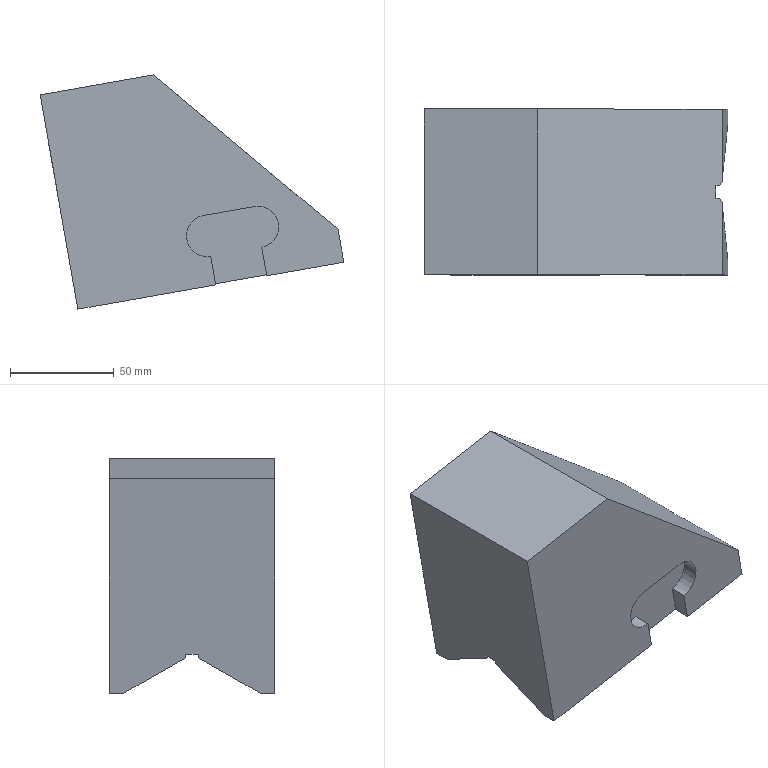Part | NX | features MAIN_BODY 2 | 1 solid | 28 faces | box 146.525 x 80 x 113.064 mm | volume 728012 mm3 | plane 24 | cylinder 4 | commonest cylinder face diameters 20 x4
STEP:
#1=CARTESIAN_POINT('',(-339.128,-33.,27.071));
#2=VERTEX_POINT('',#1);
#3=CARTESIAN_POINT('',(-339.128,-27.,27.071));
#4=VERTEX_POINT('',#3);
#5=CARTESIAN_POINT('',(-339.128,-33.,27.071));
#6=DIRECTION('',(0.,1.,0.));
#7=VECTOR('',#6,1000.);
#8=LINE('',#5,#7);
#9=EDGE_CURVE('',#2,#4,#8,.T.);
#10=ORIENTED_EDGE('',*,*,#9,.T.);
#11=CARTESIAN_POINT('',(-337.396,-27.,25.618));
#12=VERTEX_POINT('',#11);
#13=CARTESIAN_POINT('',(-336.183,-27.,24.6));
#14=DIRECTION('',(-0.766,0.,0.6428));
#15=VECTOR('',#14,1000.);
#16=LINE('',#13,#15);
#17=EDGE_CURVE('',#12,#4,#16,.T.);
#18=ORIENTED_EDGE('',*,*,#17,.F.);
#19=CARTESIAN_POINT('',(-336.183,-24.899,24.6));
#20=VERTEX_POINT('',#19);
#21=CARTESIAN_POINT('',(-337.263,-26.77,25.507));
#22=DIRECTION('',(0.4611,0.7986,-0.3869));
#23=VECTOR('',#22,1000.);
#24=LINE('',#21,#23);
#25=EDGE_CURVE('',#12,#20,#24,.T.);
#26=ORIENTED_EDGE('',*,*,#25,.T.);
#27=CARTESIAN_POINT('',(-336.183,10.,24.6));
#28=VERTEX_POINT('',#27);
#29=CARTESIAN_POINT('',(-336.183,10.,24.6));
#30=DIRECTION('',(0.,1.,0.));
#31=VECTOR('',#30,1000.);
#32=LINE('',#29,#31);
#33=EDGE_CURVE('',#20,#28,#32,.T.);
#34=ORIENTED_EDGE('',*,*,#33,.T.);
#35=CARTESIAN_POINT('',(-425.126,10.,99.232));
#36=VERTEX_POINT('',#35);
#37=CARTESIAN_POINT('',(-389.711,10.,69.515));
#38=DIRECTION('',(-0.766,0.,0.6428));
#39=VECTOR('',#38,1000.);
#40=LINE('',#37,#39);
#41=EDGE_CURVE('',#28,#36,#40,.T.);
#42=ORIENTED_EDGE('',*,*,#41,.T.);
#43=CARTESIAN_POINT('',(-425.126,-70.,99.232));
#44=VERTEX_POINT('',#43);
#45=CARTESIAN_POINT('',(-425.126,-70.,99.232));
#46=DIRECTION('',(0.,1.,0.));
#47=VECTOR('',#46,1000.);
#48=LINE('',#45,#47);
#49=EDGE_CURVE('',#44,#36,#48,.T.);
#50=ORIENTED_EDGE('',*,*,#49,.F.);
#51=CARTESIAN_POINT('',(-336.183,-70.,24.6));
#52=VERTEX_POINT('',#51);
#53=CARTESIAN_POINT('',(-389.711,-70.,69.515));
#54=DIRECTION('',(0.766,0.,-0.6428));
#55=VECTOR('',#54,1000.);
#56=LINE('',#53,#55);
#57=EDGE_CURVE('',#44,#52,#56,.T.);
#58=ORIENTED_EDGE('',*,*,#57,.T.);
#59=CARTESIAN_POINT('',(-336.183,-35.101,24.6));
#60=VERTEX_POINT('',#59);
#61=CARTESIAN_POINT('',(-336.183,10.,24.6));
#62=DIRECTION('',(0.,1.,0.));
#63=VECTOR('',#62,1000.);
#64=LINE('',#61,#63);
#65=EDGE_CURVE('',#52,#60,#64,.T.);
#66=ORIENTED_EDGE('',*,*,#65,.T.);
#67=CARTESIAN_POINT('',(-337.396,-33.,25.618));
#68=VERTEX_POINT('',#67);
#69=CARTESIAN_POINT('',(-323.333,-57.358,13.818));
#70=DIRECTION('',(0.4611,-0.7986,-0.3869));
#71=VECTOR('',#70,1000.);
#72=LINE('',#69,#71);
#73=EDGE_CURVE('',#68,#60,#72,.T.);
#74=ORIENTED_EDGE('',*,*,#73,.F.);
#75=CARTESIAN_POINT('',(-336.183,-33.,24.6));
#76=DIRECTION('',(0.766,0.,-0.6428));
#77=VECTOR('',#76,1000.);
#78=LINE('',#75,#77);
#79=EDGE_CURVE('',#2,#68,#78,.T.);
#80=ORIENTED_EDGE('',*,*,#79,.F.);
#81=EDGE_LOOP('',(#10,#18,#26,#34,#42,#50,#58,#66,#74,#80));
#82=FACE_BOUND('',#81,.T.);
#83=CARTESIAN_POINT('',(-340.414,-27.,28.15));
#84=VERTEX_POINT('',#83);
#85=CARTESIAN_POINT('',(-340.414,-33.,28.15));
#86=VERTEX_POINT('',#85);
#87=CARTESIAN_POINT('',(-340.414,-70.,28.15));
#88=DIRECTION('',(0.,-1.,0.));
#89=VECTOR('',#88,1000.);
#90=LINE('',#87,#89);
#91=EDGE_CURVE('',#84,#86,#90,.T.);
#92=ORIENTED_EDGE('',*,*,#91,.F.);
#93=ORIENTED_EDGE('',*,*,#91,.T.);
#94=EDGE_LOOP('',(#92,#93));
#95=FACE_BOUND('',#94,.T.);
#96=CARTESIAN_POINT('',(-336.183,-70.,24.6));
#97=DIRECTION('',(0.6428,0.,0.766));
#98=DIRECTION('',(-0.766,0.,0.6428));
#99=AXIS2_PLACEMENT_3D('',#96,#97,#98);
#100=PLANE('',#99);
#101=ADVANCED_FACE('',(#82,#95),#100,.T.);
#102=CARTESIAN_POINT('',(-339.967,-33.,25.165));
#103=VERTEX_POINT('',#102);
#104=CARTESIAN_POINT('',(-464.686,-33.,3.173));
#105=VERTEX_POINT('',#104);
#106=CARTESIAN_POINT('',(-336.664,-33.,25.747));
#107=DIRECTION('',(-0.9848,0.,-0.1736));
#108=VECTOR('',#107,1000.);
#109=LINE('',#106,#108);
#110=EDGE_CURVE('',#103,#105,#109,.T.);
#111=ORIENTED_EDGE('',*,*,#110,.T.);
#112=CARTESIAN_POINT('',(-464.987,-33.,4.879));
#113=VERTEX_POINT('',#112);
#114=CARTESIAN_POINT('',(-479.92,-33.,89.57));
#115=DIRECTION('',(0.1736,0.,-0.9848));
#116=VECTOR('',#115,1000.);
#117=LINE('',#114,#116);
#118=EDGE_CURVE('',#105,#113,#117,.F.);
#119=ORIENTED_EDGE('',*,*,#118,.T.);
#120=CARTESIAN_POINT('',(-336.964,-33.,27.453));
#121=DIRECTION('',(-0.9848,0.,-0.1736));
#122=VECTOR('',#121,1000.);
#123=LINE('',#120,#122);
#124=EDGE_CURVE('',#2,#113,#123,.T.);
#125=ORIENTED_EDGE('',*,*,#124,.F.);
#126=ORIENTED_EDGE('',*,*,#79,.T.);
#127=CARTESIAN_POINT('',(-336.664,-33.,25.747));
#128=DIRECTION('',(-0.9848,0.,-0.1736));
#129=VECTOR('',#128,1000.);
#130=LINE('',#127,#129);
#131=EDGE_CURVE('',#68,#103,#130,.T.);
#132=ORIENTED_EDGE('',*,*,#131,.T.);
#133=EDGE_LOOP('',(#111,#119,#125,#126,#132));
#134=FACE_BOUND('',#133,.T.);
#135=CARTESIAN_POINT('',(-336.664,-33.,25.747));
#136=DIRECTION('',(0.,1.,0.));
#137=DIRECTION('',(-0.1736,0.,0.9848));
#138=AXIS2_PLACEMENT_3D('',#135,#136,#137);
#139=PLANE('',#138);
#140=ADVANCED_FACE('',(#134),#139,.T.);
#141=ORIENTED_EDGE('',*,*,#124,.T.);
#142=CARTESIAN_POINT('',(-464.987,-27.,4.879));
#143=VERTEX_POINT('',#142);
#144=CARTESIAN_POINT('',(-464.987,-70.,4.879));
#145=DIRECTION('',(0.,-1.,0.));
#146=VECTOR('',#145,1000.);
#147=LINE('',#144,#146);
#148=EDGE_CURVE('',#113,#143,#147,.F.);
#149=ORIENTED_EDGE('',*,*,#148,.T.);
#150=CARTESIAN_POINT('',(-336.964,-27.,27.453));
#151=DIRECTION('',(-0.9848,0.,-0.1736));
#152=VECTOR('',#151,1000.);
#153=LINE('',#150,#152);
#154=EDGE_CURVE('',#4,#143,#153,.T.);
#155=ORIENTED_EDGE('',*,*,#154,.F.);
#156=ORIENTED_EDGE('',*,*,#9,.F.);
#157=EDGE_LOOP('',(#141,#149,#155,#156));
#158=FACE_BOUND('',#157,.T.);
#159=CARTESIAN_POINT('',(-336.964,-33.,27.453));
#160=DIRECTION('',(0.1736,0.,-0.9848));
#161=DIRECTION('',(0.,1.,0.));
#162=AXIS2_PLACEMENT_3D('',#159,#160,#161);
#163=PLANE('',#162);
#164=ADVANCED_FACE('',(#158),#163,.T.);
#165=ORIENTED_EDGE('',*,*,#154,.T.);
#166=CARTESIAN_POINT('',(-464.686,-27.,3.173));
#167=VERTEX_POINT('',#166);
#168=CARTESIAN_POINT('',(-479.92,-27.,89.57));
#169=DIRECTION('',(-0.1736,0.,0.9848));
#170=VECTOR('',#169,1000.);
#171=LINE('',#168,#170);
#172=EDGE_CURVE('',#143,#167,#171,.F.);
#173=ORIENTED_EDGE('',*,*,#172,.T.);
#174=CARTESIAN_POINT('',(-336.664,-27.,25.747));
#175=DIRECTION('',(-0.9848,0.,-0.1736));
#176=VECTOR('',#175,1000.);
#177=LINE('',#174,#176);
#178=EDGE_CURVE('',#12,#167,#177,.T.);
#179=ORIENTED_EDGE('',*,*,#178,.F.);
#180=ORIENTED_EDGE('',*,*,#17,.T.);
#181=EDGE_LOOP('',(#165,#173,#179,#180));
#182=FACE_BOUND('',#181,.T.);
#183=CARTESIAN_POINT('',(-336.964,-27.,27.453));
#184=DIRECTION('',(0.,-1.,0.));
#185=DIRECTION('',(0.1736,0.,-0.9848));
#186=AXIS2_PLACEMENT_3D('',#183,#184,#185);
#187=PLANE('',#186);
#188=ADVANCED_FACE('',(#182),#187,.T.);
#189=CARTESIAN_POINT('',(-333.395,10.,8.789));
#190=VERTEX_POINT('',#189);
#191=CARTESIAN_POINT('',(-342.512,10.,60.491));
#192=DIRECTION('',(0.1736,0.,-0.9848));
#193=VECTOR('',#192,1000.);
#194=LINE('',#191,#193);
#195=EDGE_CURVE('',#28,#190,#194,.T.);
#196=ORIENTED_EDGE('',*,*,#195,.T.);
#197=CARTESIAN_POINT('',(-370.595,10.,2.23));
#198=VERTEX_POINT('',#197);
#199=CARTESIAN_POINT('',(-397.678,10.,-2.546));
#200=DIRECTION('',(-0.9848,0.,-0.1736));
#201=VECTOR('',#200,1000.);
#202=LINE('',#199,#201);
#203=EDGE_CURVE('',#190,#198,#202,.T.);
#204=ORIENTED_EDGE('',*,*,#203,.T.);
#205=CARTESIAN_POINT('',(-373.026,10.,16.017));
#206=VERTEX_POINT('',#205);
#207=CARTESIAN_POINT('',(-373.026,10.,16.017));
#208=DIRECTION('',(-0.1736,0.,0.9848));
#209=VECTOR('',#208,1000.);
#210=LINE('',#207,#209);
#211=EDGE_CURVE('',#198,#206,#210,.T.);
#212=ORIENTED_EDGE('',*,*,#211,.T.);
#213=CARTESIAN_POINT('',(-376.499,10.,35.713));
#214=VERTEX_POINT('',#213);
#215=CARTESIAN_POINT('',(-374.763,10.,25.865));
#216=DIRECTION('',(0.,1.,0.));
#217=DIRECTION('',(-0.9659,0.,0.2588));
#218=AXIS2_PLACEMENT_3D('',#215,#216,#217);
#219=CIRCLE('',#218,10.);
#220=EDGE_CURVE('',#214,#206,#219,.T.);
#221=ORIENTED_EDGE('',*,*,#220,.F.);
#222=CARTESIAN_POINT('',(-401.12,10.,31.372));
#223=VERTEX_POINT('',#222);
#224=CARTESIAN_POINT('',(-401.12,10.,31.372));
#225=DIRECTION('',(0.9848,0.,0.1736));
#226=VECTOR('',#225,1000.);
#227=LINE('',#224,#226);
#228=EDGE_CURVE('',#223,#214,#227,.T.);
#229=ORIENTED_EDGE('',*,*,#228,.F.);
#230=CARTESIAN_POINT('',(-397.647,10.,11.676));
#231=VERTEX_POINT('',#230);
#232=CARTESIAN_POINT('',(-399.383,10.,21.524));
#233=DIRECTION('',(0.,1.,0.));
#234=DIRECTION('',(-0.9659,0.,0.2588));
#235=AXIS2_PLACEMENT_3D('',#232,#233,#234);
#236=CIRCLE('',#235,10.);
#237=EDGE_CURVE('',#231,#223,#236,.T.);
#238=ORIENTED_EDGE('',*,*,#237,.F.);
#239=CARTESIAN_POINT('',(-395.216,10.,-2.112));
#240=VERTEX_POINT('',#239);
#241=CARTESIAN_POINT('',(-392.437,10.,-17.868));
#242=DIRECTION('',(-0.1736,0.,0.9848));
#243=VECTOR('',#242,1000.);
#244=LINE('',#241,#243);
#245=EDGE_CURVE('',#240,#231,#244,.T.);
#246=ORIENTED_EDGE('',*,*,#245,.F.);
#247=CARTESIAN_POINT('',(-461.687,10.,-13.832));
#248=VERTEX_POINT('',#247);
#249=CARTESIAN_POINT('',(-397.678,10.,-2.546));
#250=DIRECTION('',(-0.9848,0.,-0.1736));
#251=VECTOR('',#250,1000.);
#252=LINE('',#249,#251);
#253=EDGE_CURVE('',#240,#248,#252,.T.);
#254=ORIENTED_EDGE('',*,*,#253,.T.);
#255=CARTESIAN_POINT('',(-479.92,10.,89.57));
#256=VERTEX_POINT('',#255);
#257=CARTESIAN_POINT('',(-479.92,10.,89.57));
#258=DIRECTION('',(0.1736,0.,-0.9848));
#259=VECTOR('',#258,1000.);
#260=LINE('',#257,#259);
#261=EDGE_CURVE('',#248,#256,#260,.F.);
#262=ORIENTED_EDGE('',*,*,#261,.T.);
#263=CARTESIAN_POINT('',(-479.92,10.,89.57));
#264=DIRECTION('',(0.9848,0.,0.1736));
#265=VECTOR('',#264,1000.);
#266=LINE('',#263,#265);
#267=EDGE_CURVE('',#256,#36,#266,.T.);
#268=ORIENTED_EDGE('',*,*,#267,.T.);
#269=ORIENTED_EDGE('',*,*,#41,.F.);
#270=EDGE_LOOP('',(#196,#204,#212,#221,#229,#238,#246,#254,#262,#268,#269));
#271=FACE_BOUND('',#270,.T.);
#272=CARTESIAN_POINT('',(-406.794,10.,49.157));
#273=DIRECTION('',(0.,1.,0.));
#274=DIRECTION('',(0.9848,0.,0.1736));
#275=AXIS2_PLACEMENT_3D('',#272,#273,#274);
#276=PLANE('',#275);
#277=ADVANCED_FACE('',(#271),#276,.T.);
#278=CARTESIAN_POINT('',(-395.216,2.909,-2.112));
#279=VERTEX_POINT('',#278);
#280=CARTESIAN_POINT('',(-461.687,2.909,-13.832));
#281=VERTEX_POINT('',#280);
#282=CARTESIAN_POINT('',(-333.665,2.909,8.741));
#283=DIRECTION('',(-0.9848,0.,-0.1736));
#284=VECTOR('',#283,1000.);
#285=LINE('',#282,#284);
#286=EDGE_CURVE('',#279,#281,#285,.T.);
#287=ORIENTED_EDGE('',*,*,#286,.T.);
#288=CARTESIAN_POINT('',(-461.687,10.,-13.832));
#289=DIRECTION('',(0.,1.,0.));
#290=VECTOR('',#289,1000.);
#291=LINE('',#288,#290);
#292=EDGE_CURVE('',#248,#281,#291,.F.);
#293=ORIENTED_EDGE('',*,*,#292,.F.);
#294=ORIENTED_EDGE('',*,*,#253,.F.);
#295=CARTESIAN_POINT('',(-395.216,10.,-2.112));
#296=DIRECTION('',(0.,1.,0.));
#297=VECTOR('',#296,1000.);
#298=LINE('',#295,#297);
#299=EDGE_CURVE('',#279,#240,#298,.T.);
#300=ORIENTED_EDGE('',*,*,#299,.F.);
#301=EDGE_LOOP('',(#287,#293,#294,#300));
#302=FACE_BOUND('',#301,.T.);
#303=CARTESIAN_POINT('',(-397.678,10.,-2.546));
#304=DIRECTION('',(0.1736,0.,-0.9848));
#305=DIRECTION('',(0.,1.,0.));
#306=AXIS2_PLACEMENT_3D('',#303,#304,#305);
#307=PLANE('',#306);
#308=ADVANCED_FACE('',(#302),#307,.T.);
#309=ORIENTED_EDGE('',*,*,#178,.T.);
#310=CARTESIAN_POINT('',(-471.728,-97.238,43.109));
#311=DIRECTION('',(-0.08682,-0.866,0.4924));
#312=VECTOR('',#311,1000.);
#313=LINE('',#310,#312);
#314=EDGE_CURVE('',#167,#281,#313,.F.);
#315=ORIENTED_EDGE('',*,*,#314,.T.);
#316=ORIENTED_EDGE('',*,*,#286,.F.);
#317=CARTESIAN_POINT('',(-395.307,2.,-1.595));
#318=VERTEX_POINT('',#317);
#319=CARTESIAN_POINT('',(-398.214,-27.,14.894));
#320=DIRECTION('',(0.08682,0.866,-0.4924));
#321=VECTOR('',#320,1000.);
#322=LINE('',#319,#321);
#323=EDGE_CURVE('',#318,#279,#322,.T.);
#324=ORIENTED_EDGE('',*,*,#323,.F.);
#325=CARTESIAN_POINT('',(-370.686,2.,2.746));
#326=VERTEX_POINT('',#325);
#327=CARTESIAN_POINT('',(-333.756,2.,9.258));
#328=DIRECTION('',(-0.9848,0.,-0.1736));
#329=VECTOR('',#328,1000.);
#330=LINE('',#327,#329);
#331=EDGE_CURVE('',#326,#318,#330,.T.);
#332=ORIENTED_EDGE('',*,*,#331,.F.);
#333=CARTESIAN_POINT('',(-370.595,2.909,2.23));
#334=VERTEX_POINT('',#333);
#335=CARTESIAN_POINT('',(-373.594,-27.,19.235));
#336=DIRECTION('',(0.08682,0.866,-0.4924));
#337=VECTOR('',#336,1000.);
#338=LINE('',#335,#337);
#339=EDGE_CURVE('',#326,#334,#338,.T.);
#340=ORIENTED_EDGE('',*,*,#339,.T.);
#341=CARTESIAN_POINT('',(-333.395,2.909,8.789));
#342=VERTEX_POINT('',#341);
#343=CARTESIAN_POINT('',(-333.665,2.909,8.741));
#344=DIRECTION('',(-0.9848,0.,-0.1736));
#345=VECTOR('',#344,1000.);
#346=LINE('',#343,#345);
#347=EDGE_CURVE('',#342,#334,#346,.T.);
#348=ORIENTED_EDGE('',*,*,#347,.F.);
#349=CARTESIAN_POINT('',(-336.394,-27.,25.795));
#350=DIRECTION('',(0.08682,0.866,-0.4924));
#351=VECTOR('',#350,1000.);
#352=LINE('',#349,#351);
#353=EDGE_CURVE('',#20,#342,#352,.T.);
#354=ORIENTED_EDGE('',*,*,#353,.F.);
#355=ORIENTED_EDGE('',*,*,#25,.F.);
#356=EDGE_LOOP('',(#309,#315,#316,#324,#332,#340,#348,#354,#355));
#357=FACE_BOUND('',#356,.T.);
#358=CARTESIAN_POINT('',(-336.664,-27.,25.747));
#359=DIRECTION('',(0.1504,-0.5,-0.8529));
#360=DIRECTION('',(0.08682,0.866,-0.4924));
#361=AXIS2_PLACEMENT_3D('',#358,#359,#360);
#362=PLANE('',#361);
#363=ADVANCED_FACE('',(#357),#362,.T.);
#364=CARTESIAN_POINT('',(-333.395,-62.909,8.789));
#365=VERTEX_POINT('',#364);
#366=CARTESIAN_POINT('',(-370.595,-62.909,2.23));
#367=VERTEX_POINT('',#366);
#368=CARTESIAN_POINT('',(-333.665,-62.909,8.741));
#369=DIRECTION('',(-0.9848,0.,-0.1736));
#370=VECTOR('',#369,1000.);
#371=LINE('',#368,#370);
#372=EDGE_CURVE('',#365,#367,#371,.T.);
#373=ORIENTED_EDGE('',*,*,#372,.F.);
#374=CARTESIAN_POINT('',(-333.395,-70.,8.789));
#375=VERTEX_POINT('',#374);
#376=CARTESIAN_POINT('',(-333.395,10.,8.789));
#377=DIRECTION('',(0.,-1.,0.));
#378=VECTOR('',#377,1000.);
#379=LINE('',#376,#378);
#380=EDGE_CURVE('',#365,#375,#379,.T.);
#381=ORIENTED_EDGE('',*,*,#380,.T.);
#382=CARTESIAN_POINT('',(-370.595,-70.,2.23));
#383=VERTEX_POINT('',#382);
#384=CARTESIAN_POINT('',(-397.678,-70.,-2.546));
#385=DIRECTION('',(0.9848,0.,0.1736));
#386=VECTOR('',#385,1000.);
#387=LINE('',#384,#386);
#388=EDGE_CURVE('',#383,#375,#387,.T.);
#389=ORIENTED_EDGE('',*,*,#388,.F.);
#390=CARTESIAN_POINT('',(-370.595,10.,2.23));
#391=DIRECTION('',(0.,-1.,0.));
#392=VECTOR('',#391,1000.);
#393=LINE('',#390,#392);
#394=EDGE_CURVE('',#367,#383,#393,.T.);
#395=ORIENTED_EDGE('',*,*,#394,.F.);
#396=EDGE_LOOP('',(#373,#381,#389,#395));
#397=FACE_BOUND('',#396,.T.);
#398=CARTESIAN_POINT('',(-397.678,10.,-2.546));
#399=DIRECTION('',(0.1736,0.,-0.9848));
#400=DIRECTION('',(0.,1.,0.));
#401=AXIS2_PLACEMENT_3D('',#398,#399,#400);
#402=PLANE('',#401);
#403=ADVANCED_FACE('',(#397),#402,.T.);
#404=CARTESIAN_POINT('',(-370.595,10.,2.23));
#405=DIRECTION('',(0.,1.,0.));
#406=VECTOR('',#405,1000.);
#407=LINE('',#404,#406);
#408=EDGE_CURVE('',#334,#198,#407,.T.);
#409=ORIENTED_EDGE('',*,*,#408,.T.);
#410=ORIENTED_EDGE('',*,*,#203,.F.);
#411=CARTESIAN_POINT('',(-333.395,10.,8.789));
#412=DIRECTION('',(0.,-1.,0.));
#413=VECTOR('',#412,1000.);
#414=LINE('',#411,#413);
#415=EDGE_CURVE('',#190,#342,#414,.T.);
#416=ORIENTED_EDGE('',*,*,#415,.T.);
#417=ORIENTED_EDGE('',*,*,#347,.T.);
#418=EDGE_LOOP('',(#409,#410,#416,#417));
#419=FACE_BOUND('',#418,.T.);
#420=CARTESIAN_POINT('',(-397.678,10.,-2.546));
#421=DIRECTION('',(0.1736,0.,-0.9848));
#422=DIRECTION('',(0.,1.,0.));
#423=AXIS2_PLACEMENT_3D('',#420,#421,#422);
#424=PLANE('',#423);
#425=ADVANCED_FACE('',(#419),#424,.T.);
#426=CARTESIAN_POINT('',(-395.216,-62.909,-2.112));
#427=VERTEX_POINT('',#426);
#428=CARTESIAN_POINT('',(-395.216,-70.,-2.112));
#429=VERTEX_POINT('',#428);
#430=CARTESIAN_POINT('',(-395.216,10.,-2.112));
#431=DIRECTION('',(0.,-1.,0.));
#432=VECTOR('',#431,1000.);
#433=LINE('',#430,#432);
#434=EDGE_CURVE('',#427,#429,#433,.T.);
#435=ORIENTED_EDGE('',*,*,#434,.T.);
#436=CARTESIAN_POINT('',(-461.687,-70.,-13.832));
#437=VERTEX_POINT('',#436);
#438=CARTESIAN_POINT('',(-397.678,-70.,-2.546));
#439=DIRECTION('',(0.9848,0.,0.1736));
#440=VECTOR('',#439,1000.);
#441=LINE('',#438,#440);
#442=EDGE_CURVE('',#437,#429,#441,.T.);
#443=ORIENTED_EDGE('',*,*,#442,.F.);
#444=CARTESIAN_POINT('',(-461.687,-62.909,-13.832));
#445=VERTEX_POINT('',#444);
#446=CARTESIAN_POINT('',(-461.687,10.,-13.832));
#447=DIRECTION('',(0.,1.,0.));
#448=VECTOR('',#447,1000.);
#449=LINE('',#446,#448);
#450=EDGE_CURVE('',#445,#437,#449,.F.);
#451=ORIENTED_EDGE('',*,*,#450,.F.);
#452=CARTESIAN_POINT('',(-333.665,-62.909,8.741));
#453=DIRECTION('',(-0.9848,0.,-0.1736));
#454=VECTOR('',#453,1000.);
#455=LINE('',#452,#454);
#456=EDGE_CURVE('',#427,#445,#455,.T.);
#457=ORIENTED_EDGE('',*,*,#456,.F.);
#458=EDGE_LOOP('',(#435,#443,#451,#457));
#459=FACE_BOUND('',#458,.T.);
#460=CARTESIAN_POINT('',(-397.678,10.,-2.546));
#461=DIRECTION('',(0.1736,0.,-0.9848));
#462=DIRECTION('',(0.,1.,0.));
#463=AXIS2_PLACEMENT_3D('',#460,#461,#462);
#464=PLANE('',#463);
#465=ADVANCED_FACE('',(#459),#464,.T.);
#466=ORIENTED_EDGE('',*,*,#415,.F.);
#467=ORIENTED_EDGE('',*,*,#195,.F.);
#468=ORIENTED_EDGE('',*,*,#33,.F.);
#469=ORIENTED_EDGE('',*,*,#353,.T.);
#470=EDGE_LOOP('',(#466,#467,#468,#469));
#471=FACE_BOUND('',#470,.T.);
#472=CARTESIAN_POINT('',(-342.512,10.,60.491));
#473=DIRECTION('',(0.9848,0.,0.1736));
#474=DIRECTION('',(0.,-1.,0.));
#475=AXIS2_PLACEMENT_3D('',#472,#473,#474);
#476=PLANE('',#475);
#477=ADVANCED_FACE('',(#471),#476,.T.);
#478=ORIENTED_EDGE('',*,*,#65,.F.);
#479=CARTESIAN_POINT('',(-342.512,-70.,60.491));
#480=DIRECTION('',(-0.1736,0.,0.9848));
#481=VECTOR('',#480,1000.);
#482=LINE('',#479,#481);
#483=EDGE_CURVE('',#375,#52,#482,.T.);
#484=ORIENTED_EDGE('',*,*,#483,.F.);
#485=ORIENTED_EDGE('',*,*,#380,.F.);
#486=CARTESIAN_POINT('',(-333.395,-62.909,8.789));
#487=DIRECTION('',(-0.08682,0.866,0.4924));
#488=VECTOR('',#487,1000.);
#489=LINE('',#486,#488);
#490=EDGE_CURVE('',#365,#60,#489,.T.);
#491=ORIENTED_EDGE('',*,*,#490,.T.);
#492=EDGE_LOOP('',(#478,#484,#485,#491));
#493=FACE_BOUND('',#492,.T.);
#494=CARTESIAN_POINT('',(-342.512,10.,60.491));
#495=DIRECTION('',(0.9848,0.,0.1736));
#496=DIRECTION('',(0.,-1.,0.));
#497=AXIS2_PLACEMENT_3D('',#494,#495,#496);
#498=PLANE('',#497);
#499=ADVANCED_FACE('',(#493),#498,.T.);
#500=ORIENTED_EDGE('',*,*,#261,.F.);
#501=ORIENTED_EDGE('',*,*,#292,.T.);
#502=ORIENTED_EDGE('',*,*,#314,.F.);
#503=ORIENTED_EDGE('',*,*,#172,.F.);
#504=ORIENTED_EDGE('',*,*,#148,.F.);
#505=ORIENTED_EDGE('',*,*,#118,.F.);
#506=CARTESIAN_POINT('',(-465.712,-22.762,8.994));
#507=DIRECTION('',(0.08682,-0.866,-0.4924));
#508=VECTOR('',#507,1000.);
#509=LINE('',#506,#508);
#510=EDGE_CURVE('',#445,#105,#509,.F.);
#511=ORIENTED_EDGE('',*,*,#510,.F.);
#512=ORIENTED_EDGE('',*,*,#450,.T.);
#513=CARTESIAN_POINT('',(-479.92,-70.,89.57));
#514=VERTEX_POINT('',#513);
#515=CARTESIAN_POINT('',(-479.92,-70.,89.57));
#516=DIRECTION('',(-0.1736,0.,0.9848));
#517=VECTOR('',#516,1000.);
#518=LINE('',#515,#517);
#519=EDGE_CURVE('',#514,#437,#518,.F.);
#520=ORIENTED_EDGE('',*,*,#519,.F.);
#521=CARTESIAN_POINT('',(-479.92,-70.,89.57));
#522=DIRECTION('',(0.,-1.,0.));
#523=VECTOR('',#522,1000.);
#524=LINE('',#521,#523);
#525=EDGE_CURVE('',#514,#256,#524,.F.);
#526=ORIENTED_EDGE('',*,*,#525,.T.);
#527=EDGE_LOOP('',(#500,#501,#502,#503,#504,#505,#511,#512,#520,#526));
#528=FACE_BOUND('',#527,.T.);
#529=CARTESIAN_POINT('',(-479.92,-70.,89.57));
#530=DIRECTION('',(0.9848,0.,0.1736));
#531=DIRECTION('',(0.,1.,0.));
#532=AXIS2_PLACEMENT_3D('',#529,#530,#531);
#533=PLANE('',#532);
#534=ADVANCED_FACE('',(#528),#533,.F.);
#535=ORIENTED_EDGE('',*,*,#57,.F.);
#536=CARTESIAN_POINT('',(-479.92,-70.,89.57));
#537=DIRECTION('',(0.9848,0.,0.1736));
#538=VECTOR('',#537,1000.);
#539=LINE('',#536,#538);
#540=EDGE_CURVE('',#514,#44,#539,.T.);
#541=ORIENTED_EDGE('',*,*,#540,.F.);
#542=ORIENTED_EDGE('',*,*,#519,.T.);
#543=ORIENTED_EDGE('',*,*,#442,.T.);
#544=CARTESIAN_POINT('',(-397.647,-70.,11.676));
#545=VERTEX_POINT('',#544);
#546=CARTESIAN_POINT('',(-392.437,-70.,-17.868));
#547=DIRECTION('',(-0.1736,0.,0.9848));
#548=VECTOR('',#547,1000.);
#549=LINE('',#546,#548);
#550=EDGE_CURVE('',#429,#545,#549,.T.);
#551=ORIENTED_EDGE('',*,*,#550,.T.);
#552=CARTESIAN_POINT('',(-401.12,-70.,31.372));
#553=VERTEX_POINT('',#552);
#554=CARTESIAN_POINT('',(-399.383,-70.,21.524));
#555=DIRECTION('',(0.,1.,0.));
#556=DIRECTION('',(-0.9659,0.,0.2588));
#557=AXIS2_PLACEMENT_3D('',#554,#555,#556);
#558=CIRCLE('',#557,10.);
#559=EDGE_CURVE('',#545,#553,#558,.T.);
#560=ORIENTED_EDGE('',*,*,#559,.T.);
#561=CARTESIAN_POINT('',(-376.499,-70.,35.713));
#562=VERTEX_POINT('',#561);
#563=CARTESIAN_POINT('',(-376.499,-70.,35.713));
#564=DIRECTION('',(-0.9848,0.,-0.1736));
#565=VECTOR('',#564,1000.);
#566=LINE('',#563,#565);
#567=EDGE_CURVE('',#562,#553,#566,.T.);
#568=ORIENTED_EDGE('',*,*,#567,.F.);
#569=CARTESIAN_POINT('',(-373.026,-70.,16.017));
#570=VERTEX_POINT('',#569);
#571=CARTESIAN_POINT('',(-374.763,-70.,25.865));
#572=DIRECTION('',(0.,1.,0.));
#573=DIRECTION('',(-0.9659,0.,0.2588));
#574=AXIS2_PLACEMENT_3D('',#571,#572,#573);
#575=CIRCLE('',#574,10.);
#576=EDGE_CURVE('',#562,#570,#575,.T.);
#577=ORIENTED_EDGE('',*,*,#576,.T.);
#578=CARTESIAN_POINT('',(-367.817,-70.,-13.527));
#579=DIRECTION('',(-0.1736,0.,0.9848));
#580=VECTOR('',#579,1000.);
#581=LINE('',#578,#580);
#582=EDGE_CURVE('',#383,#570,#581,.T.);
#583=ORIENTED_EDGE('',*,*,#582,.F.);
#584=ORIENTED_EDGE('',*,*,#388,.T.);
#585=ORIENTED_EDGE('',*,*,#483,.T.);
#586=EDGE_LOOP('',(#535,#541,#542,#543,#551,#560,#568,#577,#583,#584,#585));
#587=FACE_BOUND('',#586,.T.);
#588=CARTESIAN_POINT('',(-406.794,-70.,49.157));
#589=DIRECTION('',(0.,-1.,0.));
#590=DIRECTION('',(-0.9848,0.,-0.1736));
#591=AXIS2_PLACEMENT_3D('',#588,#589,#590);
#592=PLANE('',#591);
#593=ADVANCED_FACE('',(#587),#592,.T.);
#594=ORIENTED_EDGE('',*,*,#490,.F.);
#595=ORIENTED_EDGE('',*,*,#372,.T.);
#596=CARTESIAN_POINT('',(-370.686,-62.,2.746));
#597=VERTEX_POINT('',#596);
#598=CARTESIAN_POINT('',(-370.595,-62.909,2.23));
#599=DIRECTION('',(0.08682,-0.866,-0.4924));
#600=VECTOR('',#599,1000.);
#601=LINE('',#598,#600);
#602=EDGE_CURVE('',#597,#367,#601,.T.);
#603=ORIENTED_EDGE('',*,*,#602,.F.);
#604=CARTESIAN_POINT('',(-395.307,-62.,-1.595));
#605=VERTEX_POINT('',#604);
#606=CARTESIAN_POINT('',(-333.756,-62.,9.258));
#607=DIRECTION('',(0.9848,0.,0.1736));
#608=VECTOR('',#607,1000.);
#609=LINE('',#606,#608);
#610=EDGE_CURVE('',#605,#597,#609,.T.);
#611=ORIENTED_EDGE('',*,*,#610,.F.);
#612=CARTESIAN_POINT('',(-395.216,-62.909,-2.112));
#613=DIRECTION('',(0.08682,-0.866,-0.4924));
#614=VECTOR('',#613,1000.);
#615=LINE('',#612,#614);
#616=EDGE_CURVE('',#605,#427,#615,.T.);
#617=ORIENTED_EDGE('',*,*,#616,.T.);
#618=ORIENTED_EDGE('',*,*,#456,.T.);
#619=ORIENTED_EDGE('',*,*,#510,.T.);
#620=ORIENTED_EDGE('',*,*,#110,.F.);
#621=CARTESIAN_POINT('',(-337.469,-37.328,23.068));
#622=VERTEX_POINT('',#621);
#623=CARTESIAN_POINT('',(-324.685,-59.469,12.342));
#624=DIRECTION('',(-0.4611,0.7986,0.3869));
#625=VECTOR('',#624,1000.);
#626=LINE('',#623,#625);
#627=EDGE_CURVE('',#622,#103,#626,.T.);
#628=ORIENTED_EDGE('',*,*,#627,.F.);
#629=ORIENTED_EDGE('',*,*,#627,.T.);
#630=ORIENTED_EDGE('',*,*,#131,.F.);
#631=ORIENTED_EDGE('',*,*,#73,.T.);
#632=EDGE_LOOP('',(#594,#595,#603,#611,#617,#618,#619,#620,#628,#629,#630,#631));
#633=FACE_BOUND('',#632,.T.);
#634=CARTESIAN_POINT('',(-333.665,-62.909,8.741));
#635=DIRECTION('',(0.1504,0.5,-0.8529));
#636=DIRECTION('',(-0.08682,0.866,0.4924));
#637=AXIS2_PLACEMENT_3D('',#634,#635,#636);
#638=PLANE('',#637);
#639=ADVANCED_FACE('',(#633),#638,.T.);
#640=ORIENTED_EDGE('',*,*,#559,.F.);
#641=CARTESIAN_POINT('',(-397.647,-62.,11.676));
#642=VERTEX_POINT('',#641);
#643=CARTESIAN_POINT('',(-397.647,-62.,11.676));
#644=DIRECTION('',(0.,-1.,0.));
#645=VECTOR('',#644,1000.);
#646=LINE('',#643,#645);
#647=EDGE_CURVE('',#642,#545,#646,.T.);
#648=ORIENTED_EDGE('',*,*,#647,.F.);
#649=CARTESIAN_POINT('',(-401.12,-62.,31.372));
#650=VERTEX_POINT('',#649);
#651=CARTESIAN_POINT('',(-399.383,-62.,21.524));
#652=DIRECTION('',(0.,1.,0.));
#653=DIRECTION('',(-0.9659,0.,0.2588));
#654=AXIS2_PLACEMENT_3D('',#651,#652,#653);
#655=CIRCLE('',#654,10.);
#656=EDGE_CURVE('',#642,#650,#655,.T.);
#657=ORIENTED_EDGE('',*,*,#656,.T.);
#658=CARTESIAN_POINT('',(-401.12,-62.,31.372));
#659=DIRECTION('',(0.,-1.,0.));
#660=VECTOR('',#659,1000.);
#661=LINE('',#658,#660);
#662=EDGE_CURVE('',#650,#553,#661,.T.);
#663=ORIENTED_EDGE('',*,*,#662,.T.);
#664=EDGE_LOOP('',(#640,#648,#657,#663));
#665=FACE_BOUND('',#664,.T.);
#666=CARTESIAN_POINT('',(-399.383,-62.,21.524));
#667=DIRECTION('',(0.,-1.,0.));
#668=DIRECTION('',(-0.9397,0.,0.342));
#669=AXIS2_PLACEMENT_3D('',#666,#667,#668);
#670=CYLINDRICAL_SURFACE('',#669,10.);
#671=ADVANCED_FACE('',(#665),#670,.F.);
#672=ORIENTED_EDGE('',*,*,#567,.T.);
#673=ORIENTED_EDGE('',*,*,#662,.F.);
#674=CARTESIAN_POINT('',(-376.499,-62.,35.713));
#675=VERTEX_POINT('',#674);
#676=CARTESIAN_POINT('',(-376.499,-62.,35.713));
#677=DIRECTION('',(-0.9848,0.,-0.1736));
#678=VECTOR('',#677,1000.);
#679=LINE('',#676,#678);
#680=EDGE_CURVE('',#675,#650,#679,.T.);
#681=ORIENTED_EDGE('',*,*,#680,.F.);
#682=CARTESIAN_POINT('',(-376.499,-62.,35.713));
#683=DIRECTION('',(0.,-1.,0.));
#684=VECTOR('',#683,1000.);
#685=LINE('',#682,#684);
#686=EDGE_CURVE('',#675,#562,#685,.T.);
#687=ORIENTED_EDGE('',*,*,#686,.T.);
#688=EDGE_LOOP('',(#672,#673,#681,#687));
#689=FACE_BOUND('',#688,.T.);
#690=CARTESIAN_POINT('',(-376.499,-62.,35.713));
#691=DIRECTION('',(0.1736,0.,-0.9848));
#692=DIRECTION('',(-0.9848,0.,-0.1736));
#693=AXIS2_PLACEMENT_3D('',#690,#691,#692);
#694=PLANE('',#693);
#695=ADVANCED_FACE('',(#689),#694,.T.);
#696=ORIENTED_EDGE('',*,*,#576,.F.);
#697=ORIENTED_EDGE('',*,*,#686,.F.);
#698=CARTESIAN_POINT('',(-373.026,-62.,16.017));
#699=VERTEX_POINT('',#698);
#700=CARTESIAN_POINT('',(-374.763,-62.,25.865));
#701=DIRECTION('',(0.,1.,0.));
#702=DIRECTION('',(-0.9659,0.,0.2588));
#703=AXIS2_PLACEMENT_3D('',#700,#701,#702);
#704=CIRCLE('',#703,10.);
#705=EDGE_CURVE('',#675,#699,#704,.T.);
#706=ORIENTED_EDGE('',*,*,#705,.T.);
#707=CARTESIAN_POINT('',(-373.026,-62.,16.017));
#708=DIRECTION('',(0.,-1.,0.));
#709=VECTOR('',#708,1000.);
#710=LINE('',#707,#709);
#711=EDGE_CURVE('',#699,#570,#710,.T.);
#712=ORIENTED_EDGE('',*,*,#711,.T.);
#713=EDGE_LOOP('',(#696,#697,#706,#712));
#714=FACE_BOUND('',#713,.T.);
#715=CARTESIAN_POINT('',(-374.763,-62.,25.865));
#716=DIRECTION('',(0.,-1.,0.));
#717=DIRECTION('',(-0.9397,0.,0.342));
#718=AXIS2_PLACEMENT_3D('',#715,#716,#717);
#719=CYLINDRICAL_SURFACE('',#718,10.);
#720=ADVANCED_FACE('',(#714),#719,.F.);
#721=ORIENTED_EDGE('',*,*,#705,.F.);
#722=ORIENTED_EDGE('',*,*,#680,.T.);
#723=ORIENTED_EDGE('',*,*,#656,.F.);
#724=CARTESIAN_POINT('',(-392.437,-62.,-17.868));
#725=DIRECTION('',(-0.1736,0.,0.9848));
#726=VECTOR('',#725,1000.);
#727=LINE('',#724,#726);
#728=EDGE_CURVE('',#605,#642,#727,.T.);
#729=ORIENTED_EDGE('',*,*,#728,.F.);
#730=ORIENTED_EDGE('',*,*,#610,.T.);
#731=CARTESIAN_POINT('',(-367.817,-62.,-13.527));
#732=DIRECTION('',(-0.1736,0.,0.9848));
#733=VECTOR('',#732,1000.);
#734=LINE('',#731,#733);
#735=EDGE_CURVE('',#597,#699,#734,.T.);
#736=ORIENTED_EDGE('',*,*,#735,.T.);
#737=EDGE_LOOP('',(#721,#722,#723,#729,#730,#736));
#738=FACE_BOUND('',#737,.T.);
#739=CARTESIAN_POINT('',(-399.383,-62.,21.524));
#740=DIRECTION('',(0.,-1.,0.));
#741=DIRECTION('',(-0.9397,0.,0.342));
#742=AXIS2_PLACEMENT_3D('',#739,#740,#741);
#743=PLANE('',#742);
#744=ADVANCED_FACE('',(#738),#743,.T.);
#745=ORIENTED_EDGE('',*,*,#434,.F.);
#746=ORIENTED_EDGE('',*,*,#616,.F.);
#747=ORIENTED_EDGE('',*,*,#728,.T.);
#748=ORIENTED_EDGE('',*,*,#647,.T.);
#749=ORIENTED_EDGE('',*,*,#550,.F.);
#750=EDGE_LOOP('',(#745,#746,#747,#748,#749));
#751=FACE_BOUND('',#750,.T.);
#752=CARTESIAN_POINT('',(-392.437,-62.,-17.868));
#753=DIRECTION('',(-0.9848,0.,-0.1736));
#754=DIRECTION('',(-0.1736,0.,0.9848));
#755=AXIS2_PLACEMENT_3D('',#752,#753,#754);
#756=PLANE('',#755);
#757=ADVANCED_FACE('',(#751),#756,.F.);
#758=ORIENTED_EDGE('',*,*,#602,.T.);
#759=ORIENTED_EDGE('',*,*,#394,.T.);
#760=ORIENTED_EDGE('',*,*,#582,.T.);
#761=ORIENTED_EDGE('',*,*,#711,.F.);
#762=ORIENTED_EDGE('',*,*,#735,.F.);
#763=EDGE_LOOP('',(#758,#759,#760,#761,#762));
#764=FACE_BOUND('',#763,.T.);
#765=CARTESIAN_POINT('',(-367.817,-62.,-13.527));
#766=DIRECTION('',(-0.9848,0.,-0.1736));
#767=DIRECTION('',(-0.1736,0.,0.9848));
#768=AXIS2_PLACEMENT_3D('',#765,#766,#767);
#769=PLANE('',#768);
#770=ADVANCED_FACE('',(#764),#769,.T.);
#771=ORIENTED_EDGE('',*,*,#228,.T.);
#772=CARTESIAN_POINT('',(-376.499,2.,35.713));
#773=VERTEX_POINT('',#772);
#774=CARTESIAN_POINT('',(-376.499,10.,35.713));
#775=DIRECTION('',(0.,-1.,0.));
#776=VECTOR('',#775,1000.);
#777=LINE('',#774,#776);
#778=EDGE_CURVE('',#214,#773,#777,.T.);
#779=ORIENTED_EDGE('',*,*,#778,.T.);
#780=CARTESIAN_POINT('',(-401.12,2.,31.372));
#781=VERTEX_POINT('',#780);
#782=CARTESIAN_POINT('',(-401.12,2.,31.372));
#783=DIRECTION('',(0.9848,0.,0.1736));
#784=VECTOR('',#783,1000.);
#785=LINE('',#782,#784);
#786=EDGE_CURVE('',#781,#773,#785,.T.);
#787=ORIENTED_EDGE('',*,*,#786,.F.);
#788=CARTESIAN_POINT('',(-401.12,2.,31.372));
#789=DIRECTION('',(0.,1.,0.));
#790=VECTOR('',#789,1000.);
#791=LINE('',#788,#790);
#792=EDGE_CURVE('',#781,#223,#791,.T.);
#793=ORIENTED_EDGE('',*,*,#792,.T.);
#794=EDGE_LOOP('',(#771,#779,#787,#793));
#795=FACE_BOUND('',#794,.T.);
#796=CARTESIAN_POINT('',(-401.12,2.,31.372));
#797=DIRECTION('',(0.1736,0.,-0.9848));
#798=DIRECTION('',(-0.9848,0.,-0.1736));
#799=AXIS2_PLACEMENT_3D('',#796,#797,#798);
#800=PLANE('',#799);
#801=ADVANCED_FACE('',(#795),#800,.T.);
#802=CARTESIAN_POINT('',(-397.647,2.,11.676));
#803=VERTEX_POINT('',#802);
#804=CARTESIAN_POINT('',(-397.647,10.,11.676));
#805=DIRECTION('',(0.,-1.,0.));
#806=VECTOR('',#805,1000.);
#807=LINE('',#804,#806);
#808=EDGE_CURVE('',#231,#803,#807,.T.);
#809=ORIENTED_EDGE('',*,*,#808,.T.);
#810=CARTESIAN_POINT('',(-392.437,2.,-17.868));
#811=DIRECTION('',(-0.1736,0.,0.9848));
#812=VECTOR('',#811,1000.);
#813=LINE('',#810,#812);
#814=EDGE_CURVE('',#318,#803,#813,.T.);
#815=ORIENTED_EDGE('',*,*,#814,.F.);
#816=ORIENTED_EDGE('',*,*,#323,.T.);
#817=ORIENTED_EDGE('',*,*,#299,.T.);
#818=ORIENTED_EDGE('',*,*,#245,.T.);
#819=EDGE_LOOP('',(#809,#815,#816,#817,#818));
#820=FACE_BOUND('',#819,.T.);
#821=CARTESIAN_POINT('',(-392.437,2.,-17.868));
#822=DIRECTION('',(0.9848,0.,0.1736));
#823=DIRECTION('',(0.1736,0.,-0.9848));
#824=AXIS2_PLACEMENT_3D('',#821,#822,#823);
#825=PLANE('',#824);
#826=ADVANCED_FACE('',(#820),#825,.T.);
#827=ORIENTED_EDGE('',*,*,#211,.F.);
#828=ORIENTED_EDGE('',*,*,#408,.F.);
#829=ORIENTED_EDGE('',*,*,#339,.F.);
#830=CARTESIAN_POINT('',(-373.026,2.,16.017));
#831=VERTEX_POINT('',#830);
#832=CARTESIAN_POINT('',(-373.026,2.,16.017));
#833=DIRECTION('',(-0.1736,0.,0.9848));
#834=VECTOR('',#833,1000.);
#835=LINE('',#832,#834);
#836=EDGE_CURVE('',#326,#831,#835,.T.);
#837=ORIENTED_EDGE('',*,*,#836,.T.);
#838=CARTESIAN_POINT('',(-373.026,10.,16.017));
#839=DIRECTION('',(0.,-1.,0.));
#840=VECTOR('',#839,1000.);
#841=LINE('',#838,#840);
#842=EDGE_CURVE('',#206,#831,#841,.T.);
#843=ORIENTED_EDGE('',*,*,#842,.F.);
#844=EDGE_LOOP('',(#827,#828,#829,#837,#843));
#845=FACE_BOUND('',#844,.T.);
#846=CARTESIAN_POINT('',(-373.026,2.,16.017));
#847=DIRECTION('',(0.9848,0.,0.1736));
#848=DIRECTION('',(0.1736,0.,-0.9848));
#849=AXIS2_PLACEMENT_3D('',#846,#847,#848);
#850=PLANE('',#849);
#851=ADVANCED_FACE('',(#845),#850,.F.);
#852=CARTESIAN_POINT('',(-374.763,2.,25.865));
#853=DIRECTION('',(0.,1.,0.));
#854=DIRECTION('',(-0.9659,0.,0.2588));
#855=AXIS2_PLACEMENT_3D('',#852,#853,#854);
#856=CIRCLE('',#855,10.);
#857=EDGE_CURVE('',#773,#831,#856,.T.);
#858=ORIENTED_EDGE('',*,*,#857,.T.);
#859=ORIENTED_EDGE('',*,*,#836,.F.);
#860=ORIENTED_EDGE('',*,*,#331,.T.);
#861=ORIENTED_EDGE('',*,*,#814,.T.);
#862=CARTESIAN_POINT('',(-399.383,2.,21.524));
#863=DIRECTION('',(0.,1.,0.));
#864=DIRECTION('',(-0.9659,0.,0.2588));
#865=AXIS2_PLACEMENT_3D('',#862,#863,#864);
#866=CIRCLE('',#865,10.);
#867=EDGE_CURVE('',#803,#781,#866,.T.);
#868=ORIENTED_EDGE('',*,*,#867,.T.);
#869=ORIENTED_EDGE('',*,*,#786,.T.);
#870=EDGE_LOOP('',(#858,#859,#860,#861,#868,#869));
#871=FACE_BOUND('',#870,.T.);
#872=CARTESIAN_POINT('',(-404.593,2.,51.068));
#873=DIRECTION('',(0.,1.,0.));
#874=DIRECTION('',(-0.9397,0.,0.342));
#875=AXIS2_PLACEMENT_3D('',#872,#873,#874);
#876=PLANE('',#875);
#877=ADVANCED_FACE('',(#871),#876,.T.);
#878=ORIENTED_EDGE('',*,*,#857,.F.);
#879=ORIENTED_EDGE('',*,*,#778,.F.);
#880=ORIENTED_EDGE('',*,*,#220,.T.);
#881=ORIENTED_EDGE('',*,*,#842,.T.);
#882=EDGE_LOOP('',(#878,#879,#880,#881));
#883=FACE_BOUND('',#882,.T.);
#884=CARTESIAN_POINT('',(-374.763,10.,25.865));
#885=DIRECTION('',(0.,-1.,0.));
#886=DIRECTION('',(-0.9397,0.,0.342));
#887=AXIS2_PLACEMENT_3D('',#884,#885,#886);
#888=CYLINDRICAL_SURFACE('',#887,10.);
#889=ADVANCED_FACE('',(#883),#888,.F.);
#890=ORIENTED_EDGE('',*,*,#867,.F.);
#891=ORIENTED_EDGE('',*,*,#808,.F.);
#892=ORIENTED_EDGE('',*,*,#237,.T.);
#893=ORIENTED_EDGE('',*,*,#792,.F.);
#894=EDGE_LOOP('',(#890,#891,#892,#893));
#895=FACE_BOUND('',#894,.T.);
#896=CARTESIAN_POINT('',(-399.383,10.,21.524));
#897=DIRECTION('',(0.,-1.,0.));
#898=DIRECTION('',(-0.9397,0.,0.342));
#899=AXIS2_PLACEMENT_3D('',#896,#897,#898);
#900=CYLINDRICAL_SURFACE('',#899,10.);
#901=ADVANCED_FACE('',(#895),#900,.F.);
#902=ORIENTED_EDGE('',*,*,#49,.T.);
#903=ORIENTED_EDGE('',*,*,#267,.F.);
#904=ORIENTED_EDGE('',*,*,#525,.F.);
#905=ORIENTED_EDGE('',*,*,#540,.T.);
#906=EDGE_LOOP('',(#902,#903,#904,#905));
#907=FACE_BOUND('',#906,.T.);
#908=CARTESIAN_POINT('',(-479.92,-70.,89.57));
#909=DIRECTION('',(0.1736,0.,-0.9848));
#910=DIRECTION('',(0.9848,0.,0.1736));
#911=AXIS2_PLACEMENT_3D('',#908,#909,#910);
#912=PLANE('',#911);
#913=ADVANCED_FACE('',(#907),#912,.F.);
#914=CLOSED_SHELL('',(#101,#140,#164,#188,#277,#308,#363,#403,#425,#465,#477,#499,#534,#593,#639,#671,#695,#720,#744,#757,#770,#801,#826,#851,#877,#889,#901,#913));
#915=MANIFOLD_SOLID_BREP('',#914);
#916=(LENGTH_UNIT()NAMED_UNIT(*)SI_UNIT(.MILLI.,.METRE.));
#917=UNCERTAINTY_MEASURE_WITH_UNIT(LENGTH_MEASURE(0.00001),#916,'','');
#918=(NAMED_UNIT(*)PLANE_ANGLE_UNIT()SI_UNIT($,.RADIAN.));
#919=(NAMED_UNIT(*)SI_UNIT($,.STERADIAN.)SOLID_ANGLE_UNIT());
#920=(GEOMETRIC_REPRESENTATION_CONTEXT(3)GLOBAL_UNCERTAINTY_ASSIGNED_CONTEXT((#917))GLOBAL_UNIT_ASSIGNED_CONTEXT((#916,#918,#919))REPRESENTATION_CONTEXT('',''));
#921=ADVANCED_BREP_SHAPE_REPRESENTATION('',(#915),#920);